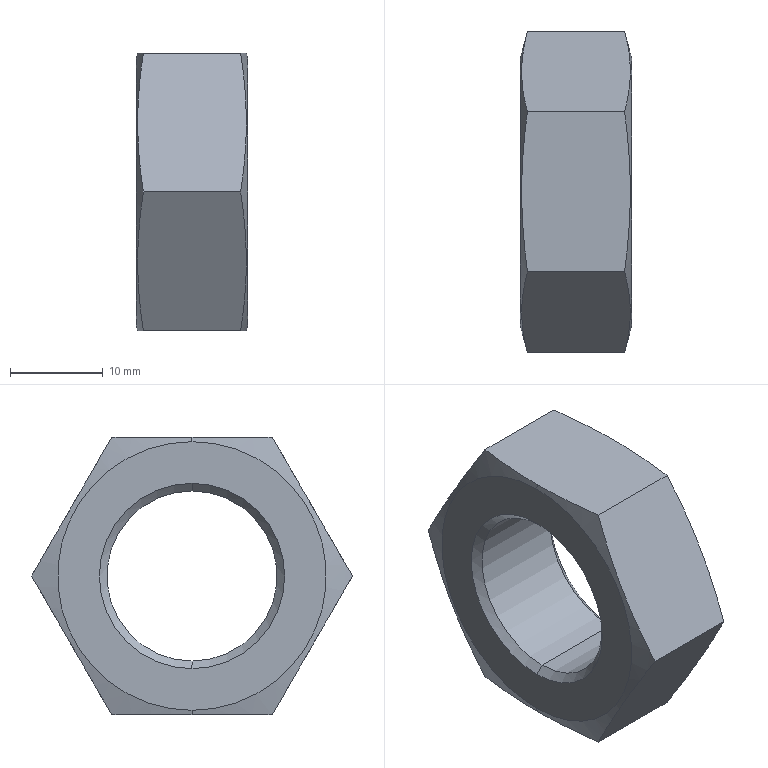Part | SolidWorks | features BaseBody 1 | 1 solid | 18 faces | box 12 x 34.641 x 30 mm | volume 6078 mm3 | cone 8 | plane 8 | cylinder 2 | commonest cylinder face diameters 18.376 x2
STEP:
#1=CARTESIAN_POINT('',(5.188,0.,9.188));
#2=VERTEX_POINT('',#1);
#3=CARTESIAN_POINT('',(5.188,0.,-9.188));
#4=VERTEX_POINT('',#3);
#5=CARTESIAN_POINT('',(5.188,0.,0.));
#6=DIRECTION('',(1.,0.,0.));
#7=DIRECTION('',(0.,0.,-1.));
#8=AXIS2_PLACEMENT_3D('',#5,#6,#7);
#9=CIRCLE('',#8,9.188);
#10=EDGE_CURVE('',#2,#4,#9,.T.);
#11=ORIENTED_EDGE('',*,*,#10,.F.);
#12=CARTESIAN_POINT('',(6.,0.,10.));
#13=VERTEX_POINT('',#12);
#14=CARTESIAN_POINT('',(6.,0.,10.));
#15=DIRECTION('',(0.7071,0.,0.7071));
#16=VECTOR('',#15,1000.);
#17=LINE('',#14,#16);
#18=EDGE_CURVE('',#2,#13,#17,.T.);
#19=ORIENTED_EDGE('',*,*,#18,.T.);
#20=CARTESIAN_POINT('',(6.,0.,-10.));
#21=VERTEX_POINT('',#20);
#22=CARTESIAN_POINT('',(6.,0.,0.));
#23=DIRECTION('',(1.,0.,0.));
#24=DIRECTION('',(0.,0.,-1.));
#25=AXIS2_PLACEMENT_3D('',#22,#23,#24);
#26=CIRCLE('',#25,10.);
#27=EDGE_CURVE('',#13,#21,#26,.T.);
#28=ORIENTED_EDGE('',*,*,#27,.T.);
#29=CARTESIAN_POINT('',(6.,0.,-10.));
#30=DIRECTION('',(0.7071,0.,-0.7071));
#31=VECTOR('',#30,1000.);
#32=LINE('',#29,#31);
#33=EDGE_CURVE('',#4,#21,#32,.T.);
#34=ORIENTED_EDGE('',*,*,#33,.F.);
#35=EDGE_LOOP('',(#11,#19,#28,#34));
#36=FACE_OUTER_BOUND('',#35,.T.);
#37=CARTESIAN_POINT('',(6.,0.,0.));
#38=DIRECTION('',(1.,0.,0.));
#39=DIRECTION('',(0.,0.,-1.));
#40=AXIS2_PLACEMENT_3D('',#37,#38,#39);
#41=CONICAL_SURFACE('',#40,10.,0.7854);
#42=ADVANCED_FACE('',(#36),#41,.F.);
#43=CARTESIAN_POINT('',(6.,0.,14.5));
#44=VERTEX_POINT('',#43);
#45=CARTESIAN_POINT('',(6.,0.,-14.5));
#46=VERTEX_POINT('',#45);
#47=CARTESIAN_POINT('',(6.,0.,0.));
#48=DIRECTION('',(-1.,0.,0.));
#49=DIRECTION('',(0.,0.,1.));
#50=AXIS2_PLACEMENT_3D('',#47,#48,#49);
#51=CIRCLE('',#50,14.5);
#52=EDGE_CURVE('',#44,#46,#51,.T.);
#53=ORIENTED_EDGE('',*,*,#52,.T.);
#54=CARTESIAN_POINT('',(5.866,0.,-15.));
#55=VERTEX_POINT('',#54);
#56=CARTESIAN_POINT('',(5.24,0.,-17.337));
#57=DIRECTION('',(-0.2588,0.,-0.9659));
#58=VECTOR('',#57,1000.);
#59=LINE('',#56,#58);
#60=EDGE_CURVE('',#46,#55,#59,.T.);
#61=ORIENTED_EDGE('',*,*,#60,.T.);
#62=CARTESIAN_POINT('',(5.244,8.66,-15.));
#63=VERTEX_POINT('',#62);
#64=CARTESIAN_POINT('',(5.866,0.,-15.));
#65=CARTESIAN_POINT('',(5.866,1.451,-15.));
#66=CARTESIAN_POINT('',(5.809,2.898,-15.));
#67=CARTESIAN_POINT('',(5.594,5.784,-15.));
#68=CARTESIAN_POINT('',(5.437,7.223,-15.));
#69=CARTESIAN_POINT('',(5.244,8.66,-15.));
#70=B_SPLINE_CURVE_WITH_KNOTS('',3,(#64,#65,#66,#67,#68,#69),.UNSPECIFIED.,.F.,.F.,(4,2,4),(0.,0.004341,0.008683),.UNSPECIFIED.);
#71=EDGE_CURVE('',#55,#63,#70,.T.);
#72=ORIENTED_EDGE('',*,*,#71,.T.);
#73=CARTESIAN_POINT('',(5.244,17.321,-0.000000051));
#74=VERTEX_POINT('',#73);
#75=CARTESIAN_POINT('',(5.244,8.66,-15.));
#76=CARTESIAN_POINT('',(5.438,9.382,-13.75));
#77=CARTESIAN_POINT('',(5.595,10.104,-12.5));
#78=CARTESIAN_POINT('',(5.809,11.547,-10.));
#79=CARTESIAN_POINT('',(5.923,12.99,-7.5));
#80=CARTESIAN_POINT('',(5.809,14.434,-5.));
#81=CARTESIAN_POINT('',(5.595,15.877,-2.5));
#82=CARTESIAN_POINT('',(5.438,16.599,-1.25));
#83=CARTESIAN_POINT('',(5.244,17.321,-0.000000051));
#84=B_SPLINE_CURVE_WITH_KNOTS('',3,(#75,#76,#77,#78,#79,#80,#81,#82,#83),.UNSPECIFIED.,.F.,.F.,(4,2,1,2,4),(0.,0.00433,0.00866,0.01299,0.01732),.UNSPECIFIED.);
#85=EDGE_CURVE('',#63,#74,#84,.T.);
#86=ORIENTED_EDGE('',*,*,#85,.T.);
#87=CARTESIAN_POINT('',(5.244,8.66,15.));
#88=VERTEX_POINT('',#87);
#89=CARTESIAN_POINT('',(5.244,17.321,-0.000000051));
#90=CARTESIAN_POINT('',(5.438,16.599,1.25));
#91=CARTESIAN_POINT('',(5.595,15.877,2.5));
#92=CARTESIAN_POINT('',(5.809,14.434,5.));
#93=CARTESIAN_POINT('',(5.923,12.99,7.5));
#94=CARTESIAN_POINT('',(5.809,11.547,10.));
#95=CARTESIAN_POINT('',(5.595,10.104,12.5));
#96=CARTESIAN_POINT('',(5.438,9.382,13.75));
#97=CARTESIAN_POINT('',(5.244,8.66,15.));
#98=B_SPLINE_CURVE_WITH_KNOTS('',3,(#89,#90,#91,#92,#93,#94,#95,#96,#97),.UNSPECIFIED.,.F.,.F.,(4,2,1,2,4),(0.,0.00433,0.00866,0.01299,0.01732),.UNSPECIFIED.);
#99=EDGE_CURVE('',#74,#88,#98,.T.);
#100=ORIENTED_EDGE('',*,*,#99,.T.);
#101=CARTESIAN_POINT('',(5.866,0.,15.));
#102=VERTEX_POINT('',#101);
#103=CARTESIAN_POINT('',(5.244,8.66,15.));
#104=CARTESIAN_POINT('',(5.437,7.223,15.));
#105=CARTESIAN_POINT('',(5.594,5.784,15.));
#106=CARTESIAN_POINT('',(5.809,2.898,15.));
#107=CARTESIAN_POINT('',(5.866,1.451,15.));
#108=CARTESIAN_POINT('',(5.866,0.,15.));
#109=B_SPLINE_CURVE_WITH_KNOTS('',3,(#103,#104,#105,#106,#107,#108),.UNSPECIFIED.,.F.,.F.,(4,2,4),(0.,0.004341,0.008683),.UNSPECIFIED.);
#110=EDGE_CURVE('',#88,#102,#109,.T.);
#111=ORIENTED_EDGE('',*,*,#110,.T.);
#112=CARTESIAN_POINT('',(5.24,0.,17.337));
#113=DIRECTION('',(-0.2588,0.,0.9659));
#114=VECTOR('',#113,1000.);
#115=LINE('',#112,#114);
#116=EDGE_CURVE('',#44,#102,#115,.T.);
#117=ORIENTED_EDGE('',*,*,#116,.F.);
#118=EDGE_LOOP('',(#53,#61,#72,#86,#100,#111,#117));
#119=FACE_OUTER_BOUND('',#118,.T.);
#120=CARTESIAN_POINT('',(5.24,0.,0.));
#121=DIRECTION('',(-1.,0.,0.));
#122=DIRECTION('',(0.,0.,1.));
#123=AXIS2_PLACEMENT_3D('',#120,#121,#122);
#124=CONICAL_SURFACE('',#123,17.337,1.309);
#125=ADVANCED_FACE('',(#119),#124,.T.);
#126=ORIENTED_EDGE('',*,*,#10,.T.);
#127=CARTESIAN_POINT('',(-5.188,0.,-9.188));
#128=VERTEX_POINT('',#127);
#129=CARTESIAN_POINT('',(6.,0.,-9.188));
#130=DIRECTION('',(-1.,0.,0.));
#131=VECTOR('',#130,1000.);
#132=LINE('',#129,#131);
#133=EDGE_CURVE('',#4,#128,#132,.T.);
#134=ORIENTED_EDGE('',*,*,#133,.T.);
#135=CARTESIAN_POINT('',(-5.188,0.,9.188));
#136=VERTEX_POINT('',#135);
#137=CARTESIAN_POINT('',(-5.188,0.,0.));
#138=DIRECTION('',(1.,0.,0.));
#139=DIRECTION('',(0.,0.,1.));
#140=AXIS2_PLACEMENT_3D('',#137,#138,#139);
#141=CIRCLE('',#140,9.188);
#142=EDGE_CURVE('',#136,#128,#141,.T.);
#143=ORIENTED_EDGE('',*,*,#142,.F.);
#144=CARTESIAN_POINT('',(6.,0.,9.188));
#145=DIRECTION('',(-1.,0.,0.));
#146=VECTOR('',#145,1000.);
#147=LINE('',#144,#146);
#148=EDGE_CURVE('',#2,#136,#147,.T.);
#149=ORIENTED_EDGE('',*,*,#148,.F.);
#150=EDGE_LOOP('',(#126,#134,#143,#149));
#151=FACE_OUTER_BOUND('',#150,.T.);
#152=CARTESIAN_POINT('',(6.,0.,0.));
#153=DIRECTION('',(-1.,0.,0.));
#154=DIRECTION('',(0.,0.,1.));
#155=AXIS2_PLACEMENT_3D('',#152,#153,#154);
#156=CYLINDRICAL_SURFACE('',#155,9.188);
#157=ADVANCED_FACE('',(#151),#156,.F.);
#158=ORIENTED_EDGE('',*,*,#142,.T.);
#159=CARTESIAN_POINT('',(-6.,0.,-10.));
#160=VERTEX_POINT('',#159);
#161=CARTESIAN_POINT('',(-6.,0.,-10.));
#162=DIRECTION('',(-0.7071,0.,-0.7071));
#163=VECTOR('',#162,1000.);
#164=LINE('',#161,#163);
#165=EDGE_CURVE('',#128,#160,#164,.T.);
#166=ORIENTED_EDGE('',*,*,#165,.T.);
#167=CARTESIAN_POINT('',(-6.,0.,10.));
#168=VERTEX_POINT('',#167);
#169=CARTESIAN_POINT('',(-6.,0.,0.));
#170=DIRECTION('',(1.,0.,0.));
#171=DIRECTION('',(0.,0.,1.));
#172=AXIS2_PLACEMENT_3D('',#169,#170,#171);
#173=CIRCLE('',#172,10.);
#174=EDGE_CURVE('',#168,#160,#173,.T.);
#175=ORIENTED_EDGE('',*,*,#174,.F.);
#176=CARTESIAN_POINT('',(-6.,0.,10.));
#177=DIRECTION('',(-0.7071,0.,0.7071));
#178=VECTOR('',#177,1000.);
#179=LINE('',#176,#178);
#180=EDGE_CURVE('',#136,#168,#179,.T.);
#181=ORIENTED_EDGE('',*,*,#180,.F.);
#182=EDGE_LOOP('',(#158,#166,#175,#181));
#183=FACE_OUTER_BOUND('',#182,.T.);
#184=CARTESIAN_POINT('',(-6.,0.,0.));
#185=DIRECTION('',(-1.,0.,0.));
#186=DIRECTION('',(0.,0.,1.));
#187=AXIS2_PLACEMENT_3D('',#184,#185,#186);
#188=CONICAL_SURFACE('',#187,10.,0.7854);
#189=ADVANCED_FACE('',(#183),#188,.F.);
#190=CARTESIAN_POINT('',(-6.,0.,-14.5));
#191=VERTEX_POINT('',#190);
#192=CARTESIAN_POINT('',(-6.,0.,14.5));
#193=VERTEX_POINT('',#192);
#194=CARTESIAN_POINT('',(-6.,0.,0.));
#195=DIRECTION('',(1.,0.,0.));
#196=DIRECTION('',(0.,0.,-1.));
#197=AXIS2_PLACEMENT_3D('',#194,#195,#196);
#198=CIRCLE('',#197,14.5);
#199=EDGE_CURVE('',#191,#193,#198,.T.);
#200=ORIENTED_EDGE('',*,*,#199,.T.);
#201=CARTESIAN_POINT('',(-5.866,0.,15.));
#202=VERTEX_POINT('',#201);
#203=CARTESIAN_POINT('',(-5.24,0.,17.337));
#204=DIRECTION('',(0.2588,0.,0.9659));
#205=VECTOR('',#204,1000.);
#206=LINE('',#203,#205);
#207=EDGE_CURVE('',#193,#202,#206,.T.);
#208=ORIENTED_EDGE('',*,*,#207,.T.);
#209=CARTESIAN_POINT('',(-5.244,8.66,15.));
#210=VERTEX_POINT('',#209);
#211=CARTESIAN_POINT('',(-5.866,0.,15.));
#212=CARTESIAN_POINT('',(-5.866,1.451,15.));
#213=CARTESIAN_POINT('',(-5.809,2.898,15.));
#214=CARTESIAN_POINT('',(-5.594,5.784,15.));
#215=CARTESIAN_POINT('',(-5.437,7.223,15.));
#216=CARTESIAN_POINT('',(-5.244,8.66,15.));
#217=B_SPLINE_CURVE_WITH_KNOTS('',3,(#211,#212,#213,#214,#215,#216),.UNSPECIFIED.,.F.,.F.,(4,2,4),(0.,0.004341,0.008683),.UNSPECIFIED.);
#218=EDGE_CURVE('',#202,#210,#217,.T.);
#219=ORIENTED_EDGE('',*,*,#218,.T.);
#220=CARTESIAN_POINT('',(-5.244,17.321,0.));
#221=VERTEX_POINT('',#220);
#222=CARTESIAN_POINT('',(-5.244,8.66,15.));
#223=CARTESIAN_POINT('',(-5.438,9.382,13.75));
#224=CARTESIAN_POINT('',(-5.595,10.104,12.5));
#225=CARTESIAN_POINT('',(-5.809,11.547,10.));
#226=CARTESIAN_POINT('',(-5.923,12.99,7.5));
#227=CARTESIAN_POINT('',(-5.809,14.434,5.));
#228=CARTESIAN_POINT('',(-5.595,15.877,2.5));
#229=CARTESIAN_POINT('',(-5.438,16.599,1.25));
#230=CARTESIAN_POINT('',(-5.244,17.321,0.));
#231=B_SPLINE_CURVE_WITH_KNOTS('',3,(#222,#223,#224,#225,#226,#227,#228,#229,#230),.UNSPECIFIED.,.F.,.F.,(4,2,1,2,4),(0.,0.00433,0.00866,0.01299,0.01732),.UNSPECIFIED.);
#232=EDGE_CURVE('',#210,#221,#231,.T.);
#233=ORIENTED_EDGE('',*,*,#232,.T.);
#234=CARTESIAN_POINT('',(-5.244,8.66,-15.));
#235=VERTEX_POINT('',#234);
#236=CARTESIAN_POINT('',(-5.244,17.321,0.));
#237=CARTESIAN_POINT('',(-5.438,16.599,-1.25));
#238=CARTESIAN_POINT('',(-5.595,15.877,-2.5));
#239=CARTESIAN_POINT('',(-5.809,14.434,-5.));
#240=CARTESIAN_POINT('',(-5.923,12.99,-7.5));
#241=CARTESIAN_POINT('',(-5.809,11.547,-10.));
#242=CARTESIAN_POINT('',(-5.595,10.104,-12.5));
#243=CARTESIAN_POINT('',(-5.438,9.382,-13.75));
#244=CARTESIAN_POINT('',(-5.244,8.66,-15.));
#245=B_SPLINE_CURVE_WITH_KNOTS('',3,(#236,#237,#238,#239,#240,#241,#242,#243,#244),.UNSPECIFIED.,.F.,.F.,(4,2,1,2,4),(0.,0.00433,0.00866,0.01299,0.01732),.UNSPECIFIED.);
#246=EDGE_CURVE('',#221,#235,#245,.T.);
#247=ORIENTED_EDGE('',*,*,#246,.T.);
#248=CARTESIAN_POINT('',(-5.866,0.,-15.));
#249=VERTEX_POINT('',#248);
#250=CARTESIAN_POINT('',(-5.244,8.66,-15.));
#251=CARTESIAN_POINT('',(-5.437,7.223,-15.));
#252=CARTESIAN_POINT('',(-5.594,5.784,-15.));
#253=CARTESIAN_POINT('',(-5.809,2.898,-15.));
#254=CARTESIAN_POINT('',(-5.866,1.451,-15.));
#255=CARTESIAN_POINT('',(-5.866,0.,-15.));
#256=B_SPLINE_CURVE_WITH_KNOTS('',3,(#250,#251,#252,#253,#254,#255),.UNSPECIFIED.,.F.,.F.,(4,2,4),(-0.008683,-0.004341,0.),.UNSPECIFIED.);
#257=EDGE_CURVE('',#235,#249,#256,.T.);
#258=ORIENTED_EDGE('',*,*,#257,.T.);
#259=CARTESIAN_POINT('',(-5.24,0.,-17.337));
#260=DIRECTION('',(0.2588,0.,-0.9659));
#261=VECTOR('',#260,1000.);
#262=LINE('',#259,#261);
#263=EDGE_CURVE('',#191,#249,#262,.T.);
#264=ORIENTED_EDGE('',*,*,#263,.F.);
#265=EDGE_LOOP('',(#200,#208,#219,#233,#247,#258,#264));
#266=FACE_OUTER_BOUND('',#265,.T.);
#267=CARTESIAN_POINT('',(-5.24,0.,0.));
#268=DIRECTION('',(1.,0.,0.));
#269=DIRECTION('',(0.,0.,-1.));
#270=AXIS2_PLACEMENT_3D('',#267,#268,#269);
#271=CONICAL_SURFACE('',#270,17.337,1.309);
#272=ADVANCED_FACE('',(#266),#271,.T.);
#273=CARTESIAN_POINT('',(6.,0.,0.));
#274=DIRECTION('',(1.,0.,0.));
#275=DIRECTION('',(0.,0.,-1.));
#276=AXIS2_PLACEMENT_3D('',#273,#274,#275);
#277=CIRCLE('',#276,10.);
#278=EDGE_CURVE('',#21,#13,#277,.T.);
#279=ORIENTED_EDGE('',*,*,#278,.F.);
#280=ORIENTED_EDGE('',*,*,#27,.F.);
#281=EDGE_LOOP('',(#279,#280));
#282=FACE_BOUND('',#281,.T.);
#283=ORIENTED_EDGE('',*,*,#52,.F.);
#284=CARTESIAN_POINT('',(6.,0.,0.));
#285=DIRECTION('',(-1.,0.,0.));
#286=DIRECTION('',(0.,0.,1.));
#287=AXIS2_PLACEMENT_3D('',#284,#285,#286);
#288=CIRCLE('',#287,14.5);
#289=EDGE_CURVE('',#46,#44,#288,.T.);
#290=ORIENTED_EDGE('',*,*,#289,.F.);
#291=EDGE_LOOP('',(#283,#290));
#292=FACE_OUTER_BOUND('',#291,.T.);
#293=CARTESIAN_POINT('',(6.,10.,0.));
#294=DIRECTION('',(-1.,0.,0.));
#295=DIRECTION('',(0.,0.,1.));
#296=AXIS2_PLACEMENT_3D('',#293,#294,#295);
#297=PLANE('',#296);
#298=ADVANCED_FACE('',(#282,#292),#297,.F.);
#299=ORIENTED_EDGE('',*,*,#18,.F.);
#300=CARTESIAN_POINT('',(5.188,0.,0.));
#301=DIRECTION('',(1.,0.,0.));
#302=DIRECTION('',(0.,0.,-1.));
#303=AXIS2_PLACEMENT_3D('',#300,#301,#302);
#304=CIRCLE('',#303,9.188);
#305=EDGE_CURVE('',#4,#2,#304,.T.);
#306=ORIENTED_EDGE('',*,*,#305,.F.);
#307=ORIENTED_EDGE('',*,*,#33,.T.);
#308=ORIENTED_EDGE('',*,*,#278,.T.);
#309=EDGE_LOOP('',(#299,#306,#307,#308));
#310=FACE_OUTER_BOUND('',#309,.T.);
#311=CARTESIAN_POINT('',(6.,0.,0.));
#312=DIRECTION('',(1.,0.,0.));
#313=DIRECTION('',(0.,0.,-1.));
#314=AXIS2_PLACEMENT_3D('',#311,#312,#313);
#315=CONICAL_SURFACE('',#314,10.,0.7854);
#316=ADVANCED_FACE('',(#310),#315,.F.);
#317=ORIENTED_EDGE('',*,*,#60,.F.);
#318=ORIENTED_EDGE('',*,*,#289,.T.);
#319=ORIENTED_EDGE('',*,*,#116,.T.);
#320=CARTESIAN_POINT('',(5.244,-8.66,15.));
#321=VERTEX_POINT('',#320);
#322=CARTESIAN_POINT('',(5.866,0.,15.));
#323=CARTESIAN_POINT('',(5.866,-1.451,15.));
#324=CARTESIAN_POINT('',(5.809,-2.898,15.));
#325=CARTESIAN_POINT('',(5.594,-5.784,15.));
#326=CARTESIAN_POINT('',(5.437,-7.223,15.));
#327=CARTESIAN_POINT('',(5.244,-8.66,15.));
#328=B_SPLINE_CURVE_WITH_KNOTS('',3,(#322,#323,#324,#325,#326,#327),.UNSPECIFIED.,.F.,.F.,(4,2,4),(0.008683,0.01302,0.01737),.UNSPECIFIED.);
#329=EDGE_CURVE('',#102,#321,#328,.T.);
#330=ORIENTED_EDGE('',*,*,#329,.T.);
#331=CARTESIAN_POINT('',(5.244,-17.321,0.000000051));
#332=VERTEX_POINT('',#331);
#333=CARTESIAN_POINT('',(5.244,-8.66,15.));
#334=CARTESIAN_POINT('',(5.438,-9.382,13.75));
#335=CARTESIAN_POINT('',(5.595,-10.104,12.5));
#336=CARTESIAN_POINT('',(5.809,-11.547,10.));
#337=CARTESIAN_POINT('',(5.923,-12.99,7.5));
#338=CARTESIAN_POINT('',(5.809,-14.434,5.));
#339=CARTESIAN_POINT('',(5.595,-15.877,2.5));
#340=CARTESIAN_POINT('',(5.438,-16.599,1.25));
#341=CARTESIAN_POINT('',(5.244,-17.321,0.000000051));
#342=B_SPLINE_CURVE_WITH_KNOTS('',3,(#333,#334,#335,#336,#337,#338,#339,#340,#341),.UNSPECIFIED.,.F.,.F.,(4,2,1,2,4),(0.,0.00433,0.00866,0.01299,0.01732),.UNSPECIFIED.);
#343=EDGE_CURVE('',#321,#332,#342,.T.);
#344=ORIENTED_EDGE('',*,*,#343,.T.);
#345=CARTESIAN_POINT('',(5.244,-8.66,-15.));
#346=VERTEX_POINT('',#345);
#347=CARTESIAN_POINT('',(5.244,-17.321,0.000000051));
#348=CARTESIAN_POINT('',(5.438,-16.599,-1.25));
#349=CARTESIAN_POINT('',(5.595,-15.877,-2.5));
#350=CARTESIAN_POINT('',(5.809,-14.434,-5.));
#351=CARTESIAN_POINT('',(5.923,-12.99,-7.5));
#352=CARTESIAN_POINT('',(5.809,-11.547,-10.));
#353=CARTESIAN_POINT('',(5.595,-10.104,-12.5));
#354=CARTESIAN_POINT('',(5.438,-9.382,-13.75));
#355=CARTESIAN_POINT('',(5.244,-8.66,-15.));
#356=B_SPLINE_CURVE_WITH_KNOTS('',3,(#347,#348,#349,#350,#351,#352,#353,#354,#355),.UNSPECIFIED.,.F.,.F.,(4,2,1,2,4),(0.,0.00433,0.00866,0.01299,0.01732),.UNSPECIFIED.);
#357=EDGE_CURVE('',#332,#346,#356,.T.);
#358=ORIENTED_EDGE('',*,*,#357,.T.);
#359=CARTESIAN_POINT('',(5.244,-8.66,-15.));
#360=CARTESIAN_POINT('',(5.437,-7.223,-15.));
#361=CARTESIAN_POINT('',(5.594,-5.784,-15.));
#362=CARTESIAN_POINT('',(5.809,-2.898,-15.));
#363=CARTESIAN_POINT('',(5.866,-1.451,-15.));
#364=CARTESIAN_POINT('',(5.866,0.,-15.));
#365=B_SPLINE_CURVE_WITH_KNOTS('',3,(#359,#360,#361,#362,#363,#364),.UNSPECIFIED.,.F.,.F.,(4,2,4),(-0.008683,-0.004341,0.),.UNSPECIFIED.);
#366=EDGE_CURVE('',#346,#55,#365,.T.);
#367=ORIENTED_EDGE('',*,*,#366,.T.);
#368=EDGE_LOOP('',(#317,#318,#319,#330,#344,#358,#367));
#369=FACE_OUTER_BOUND('',#368,.T.);
#370=CARTESIAN_POINT('',(5.24,0.,0.));
#371=DIRECTION('',(-1.,0.,0.));
#372=DIRECTION('',(0.,0.,1.));
#373=AXIS2_PLACEMENT_3D('',#370,#371,#372);
#374=CONICAL_SURFACE('',#373,17.337,1.309);
#375=ADVANCED_FACE('',(#369),#374,.T.);
#376=ORIENTED_EDGE('',*,*,#133,.F.);
#377=ORIENTED_EDGE('',*,*,#305,.T.);
#378=ORIENTED_EDGE('',*,*,#148,.T.);
#379=CARTESIAN_POINT('',(-5.188,0.,0.));
#380=DIRECTION('',(1.,0.,0.));
#381=DIRECTION('',(0.,0.,1.));
#382=AXIS2_PLACEMENT_3D('',#379,#380,#381);
#383=CIRCLE('',#382,9.188);
#384=EDGE_CURVE('',#128,#136,#383,.T.);
#385=ORIENTED_EDGE('',*,*,#384,.F.);
#386=EDGE_LOOP('',(#376,#377,#378,#385));
#387=FACE_OUTER_BOUND('',#386,.T.);
#388=CARTESIAN_POINT('',(6.,0.,0.));
#389=DIRECTION('',(-1.,0.,0.));
#390=DIRECTION('',(0.,0.,1.));
#391=AXIS2_PLACEMENT_3D('',#388,#389,#390);
#392=CYLINDRICAL_SURFACE('',#391,9.188);
#393=ADVANCED_FACE('',(#387),#392,.F.);
#394=CARTESIAN_POINT('',(-5.244,-8.66,15.));
#395=VERTEX_POINT('',#394);
#396=CARTESIAN_POINT('',(6.,-8.66,15.));
#397=DIRECTION('',(-1.,0.,0.));
#398=VECTOR('',#397,1000.);
#399=LINE('',#396,#398);
#400=EDGE_CURVE('',#321,#395,#399,.T.);
#401=ORIENTED_EDGE('',*,*,#400,.F.);
#402=ORIENTED_EDGE('',*,*,#329,.F.);
#403=ORIENTED_EDGE('',*,*,#110,.F.);
#404=CARTESIAN_POINT('',(6.,8.66,15.));
#405=DIRECTION('',(1.,0.,0.));
#406=VECTOR('',#405,1000.);
#407=LINE('',#404,#406);
#408=EDGE_CURVE('',#210,#88,#407,.T.);
#409=ORIENTED_EDGE('',*,*,#408,.F.);
#410=ORIENTED_EDGE('',*,*,#218,.F.);
#411=CARTESIAN_POINT('',(-5.244,-8.66,15.));
#412=CARTESIAN_POINT('',(-5.437,-7.223,15.));
#413=CARTESIAN_POINT('',(-5.594,-5.784,15.));
#414=CARTESIAN_POINT('',(-5.809,-2.898,15.));
#415=CARTESIAN_POINT('',(-5.866,-1.451,15.));
#416=CARTESIAN_POINT('',(-5.866,0.,15.));
#417=B_SPLINE_CURVE_WITH_KNOTS('',3,(#411,#412,#413,#414,#415,#416),.UNSPECIFIED.,.F.,.F.,(4,2,4),(-0.008683,-0.004341,0.),.UNSPECIFIED.);
#418=EDGE_CURVE('',#395,#202,#417,.T.);
#419=ORIENTED_EDGE('',*,*,#418,.F.);
#420=EDGE_LOOP('',(#401,#402,#403,#409,#410,#419));
#421=FACE_OUTER_BOUND('',#420,.T.);
#422=CARTESIAN_POINT('',(6.,8.66,15.));
#423=DIRECTION('',(0.,0.,-1.));
#424=DIRECTION('',(-1.,0.,0.));
#425=AXIS2_PLACEMENT_3D('',#422,#423,#424);
#426=PLANE('',#425);
#427=ADVANCED_FACE('',(#421),#426,.F.);
#428=ORIENTED_EDGE('',*,*,#99,.F.);
#429=CARTESIAN_POINT('',(6.,17.321,0.));
#430=DIRECTION('',(1.,0.,0.));
#431=VECTOR('',#430,1000.);
#432=LINE('',#429,#431);
#433=EDGE_CURVE('',#221,#74,#432,.T.);
#434=ORIENTED_EDGE('',*,*,#433,.F.);
#435=ORIENTED_EDGE('',*,*,#232,.F.);
#436=ORIENTED_EDGE('',*,*,#408,.T.);
#437=EDGE_LOOP('',(#428,#434,#435,#436));
#438=FACE_OUTER_BOUND('',#437,.T.);
#439=CARTESIAN_POINT('',(6.,17.321,0.));
#440=DIRECTION('',(0.,-0.866,-0.5));
#441=DIRECTION('',(0.,0.5,-0.866));
#442=AXIS2_PLACEMENT_3D('',#439,#440,#441);
#443=PLANE('',#442);
#444=ADVANCED_FACE('',(#438),#443,.F.);
#445=ORIENTED_EDGE('',*,*,#85,.F.);
#446=CARTESIAN_POINT('',(6.,8.66,-15.));
#447=DIRECTION('',(1.,0.,0.));
#448=VECTOR('',#447,1000.);
#449=LINE('',#446,#448);
#450=EDGE_CURVE('',#235,#63,#449,.T.);
#451=ORIENTED_EDGE('',*,*,#450,.F.);
#452=ORIENTED_EDGE('',*,*,#246,.F.);
#453=ORIENTED_EDGE('',*,*,#433,.T.);
#454=EDGE_LOOP('',(#445,#451,#452,#453));
#455=FACE_OUTER_BOUND('',#454,.T.);
#456=CARTESIAN_POINT('',(6.,8.66,-15.));
#457=DIRECTION('',(0.,-0.866,0.5));
#458=DIRECTION('',(0.,-0.5,-0.866));
#459=AXIS2_PLACEMENT_3D('',#456,#457,#458);
#460=PLANE('',#459);
#461=ADVANCED_FACE('',(#455),#460,.F.);
#462=ORIENTED_EDGE('',*,*,#366,.F.);
#463=CARTESIAN_POINT('',(-5.244,-8.66,-15.));
#464=VERTEX_POINT('',#463);
#465=CARTESIAN_POINT('',(6.,-8.66,-15.));
#466=DIRECTION('',(1.,0.,0.));
#467=VECTOR('',#466,1000.);
#468=LINE('',#465,#467);
#469=EDGE_CURVE('',#464,#346,#468,.T.);
#470=ORIENTED_EDGE('',*,*,#469,.F.);
#471=CARTESIAN_POINT('',(-5.866,0.,-15.));
#472=CARTESIAN_POINT('',(-5.866,-1.451,-15.));
#473=CARTESIAN_POINT('',(-5.809,-2.898,-15.));
#474=CARTESIAN_POINT('',(-5.594,-5.784,-15.));
#475=CARTESIAN_POINT('',(-5.437,-7.223,-15.));
#476=CARTESIAN_POINT('',(-5.244,-8.66,-15.));
#477=B_SPLINE_CURVE_WITH_KNOTS('',3,(#471,#472,#473,#474,#475,#476),.UNSPECIFIED.,.F.,.F.,(4,2,4),(0.,0.004341,0.008683),.UNSPECIFIED.);
#478=EDGE_CURVE('',#249,#464,#477,.T.);
#479=ORIENTED_EDGE('',*,*,#478,.F.);
#480=ORIENTED_EDGE('',*,*,#257,.F.);
#481=ORIENTED_EDGE('',*,*,#450,.T.);
#482=ORIENTED_EDGE('',*,*,#71,.F.);
#483=EDGE_LOOP('',(#462,#470,#479,#480,#481,#482));
#484=FACE_OUTER_BOUND('',#483,.T.);
#485=CARTESIAN_POINT('',(6.,-8.66,-15.));
#486=DIRECTION('',(0.,0.,1.));
#487=DIRECTION('',(1.,0.,0.));
#488=AXIS2_PLACEMENT_3D('',#485,#486,#487);
#489=PLANE('',#488);
#490=ADVANCED_FACE('',(#484),#489,.F.);
#491=ORIENTED_EDGE('',*,*,#357,.F.);
#492=CARTESIAN_POINT('',(-5.244,-17.321,0.));
#493=VERTEX_POINT('',#492);
#494=CARTESIAN_POINT('',(6.,-17.321,0.));
#495=DIRECTION('',(1.,0.,0.));
#496=VECTOR('',#495,1000.);
#497=LINE('',#494,#496);
#498=EDGE_CURVE('',#493,#332,#497,.T.);
#499=ORIENTED_EDGE('',*,*,#498,.F.);
#500=CARTESIAN_POINT('',(-5.244,-8.66,-15.));
#501=CARTESIAN_POINT('',(-5.438,-9.382,-13.75));
#502=CARTESIAN_POINT('',(-5.595,-10.104,-12.5));
#503=CARTESIAN_POINT('',(-5.809,-11.547,-10.));
#504=CARTESIAN_POINT('',(-5.923,-12.99,-7.5));
#505=CARTESIAN_POINT('',(-5.809,-14.434,-5.));
#506=CARTESIAN_POINT('',(-5.595,-15.877,-2.5));
#507=CARTESIAN_POINT('',(-5.438,-16.599,-1.25));
#508=CARTESIAN_POINT('',(-5.244,-17.321,0.));
#509=B_SPLINE_CURVE_WITH_KNOTS('',3,(#500,#501,#502,#503,#504,#505,#506,#507,#508),.UNSPECIFIED.,.F.,.F.,(4,2,1,2,4),(0.,0.00433,0.00866,0.01299,0.01732),.UNSPECIFIED.);
#510=EDGE_CURVE('',#464,#493,#509,.T.);
#511=ORIENTED_EDGE('',*,*,#510,.F.);
#512=ORIENTED_EDGE('',*,*,#469,.T.);
#513=EDGE_LOOP('',(#491,#499,#511,#512));
#514=FACE_OUTER_BOUND('',#513,.T.);
#515=CARTESIAN_POINT('',(6.,-17.321,0.));
#516=DIRECTION('',(0.,0.866,0.5));
#517=DIRECTION('',(0.,-0.5,0.866));
#518=AXIS2_PLACEMENT_3D('',#515,#516,#517);
#519=PLANE('',#518);
#520=ADVANCED_FACE('',(#514),#519,.F.);
#521=ORIENTED_EDGE('',*,*,#343,.F.);
#522=ORIENTED_EDGE('',*,*,#400,.T.);
#523=CARTESIAN_POINT('',(-5.244,-17.321,0.));
#524=CARTESIAN_POINT('',(-5.438,-16.599,1.25));
#525=CARTESIAN_POINT('',(-5.595,-15.877,2.5));
#526=CARTESIAN_POINT('',(-5.809,-14.434,5.));
#527=CARTESIAN_POINT('',(-5.923,-12.99,7.5));
#528=CARTESIAN_POINT('',(-5.809,-11.547,10.));
#529=CARTESIAN_POINT('',(-5.595,-10.104,12.5));
#530=CARTESIAN_POINT('',(-5.438,-9.382,13.75));
#531=CARTESIAN_POINT('',(-5.244,-8.66,15.));
#532=B_SPLINE_CURVE_WITH_KNOTS('',3,(#523,#524,#525,#526,#527,#528,#529,#530,#531),.UNSPECIFIED.,.F.,.F.,(4,2,1,2,4),(0.,0.00433,0.00866,0.01299,0.01732),.UNSPECIFIED.);
#533=EDGE_CURVE('',#493,#395,#532,.T.);
#534=ORIENTED_EDGE('',*,*,#533,.F.);
#535=ORIENTED_EDGE('',*,*,#498,.T.);
#536=EDGE_LOOP('',(#521,#522,#534,#535));
#537=FACE_OUTER_BOUND('',#536,.T.);
#538=CARTESIAN_POINT('',(6.,-8.66,15.));
#539=DIRECTION('',(0.,0.866,-0.5));
#540=DIRECTION('',(0.,0.5,0.866));
#541=AXIS2_PLACEMENT_3D('',#538,#539,#540);
#542=PLANE('',#541);
#543=ADVANCED_FACE('',(#537),#542,.F.);
#544=ORIENTED_EDGE('',*,*,#165,.F.);
#545=ORIENTED_EDGE('',*,*,#384,.T.);
#546=ORIENTED_EDGE('',*,*,#180,.T.);
#547=CARTESIAN_POINT('',(-6.,0.,0.));
#548=DIRECTION('',(1.,0.,0.));
#549=DIRECTION('',(0.,0.,1.));
#550=AXIS2_PLACEMENT_3D('',#547,#548,#549);
#551=CIRCLE('',#550,10.);
#552=EDGE_CURVE('',#160,#168,#551,.T.);
#553=ORIENTED_EDGE('',*,*,#552,.F.);
#554=EDGE_LOOP('',(#544,#545,#546,#553));
#555=FACE_OUTER_BOUND('',#554,.T.);
#556=CARTESIAN_POINT('',(-6.,0.,0.));
#557=DIRECTION('',(-1.,0.,0.));
#558=DIRECTION('',(0.,0.,1.));
#559=AXIS2_PLACEMENT_3D('',#556,#557,#558);
#560=CONICAL_SURFACE('',#559,10.,0.7854);
#561=ADVANCED_FACE('',(#555),#560,.F.);
#562=ORIENTED_EDGE('',*,*,#207,.F.);
#563=CARTESIAN_POINT('',(-6.,0.,0.));
#564=DIRECTION('',(1.,0.,0.));
#565=DIRECTION('',(0.,0.,-1.));
#566=AXIS2_PLACEMENT_3D('',#563,#564,#565);
#567=CIRCLE('',#566,14.5);
#568=EDGE_CURVE('',#193,#191,#567,.T.);
#569=ORIENTED_EDGE('',*,*,#568,.T.);
#570=ORIENTED_EDGE('',*,*,#263,.T.);
#571=ORIENTED_EDGE('',*,*,#478,.T.);
#572=ORIENTED_EDGE('',*,*,#510,.T.);
#573=ORIENTED_EDGE('',*,*,#533,.T.);
#574=ORIENTED_EDGE('',*,*,#418,.T.);
#575=EDGE_LOOP('',(#562,#569,#570,#571,#572,#573,#574));
#576=FACE_OUTER_BOUND('',#575,.T.);
#577=CARTESIAN_POINT('',(-5.24,0.,0.));
#578=DIRECTION('',(1.,0.,0.));
#579=DIRECTION('',(0.,0.,-1.));
#580=AXIS2_PLACEMENT_3D('',#577,#578,#579);
#581=CONICAL_SURFACE('',#580,17.337,1.309);
#582=ADVANCED_FACE('',(#576),#581,.T.);
#583=ORIENTED_EDGE('',*,*,#199,.F.);
#584=ORIENTED_EDGE('',*,*,#568,.F.);
#585=EDGE_LOOP('',(#583,#584));
#586=FACE_OUTER_BOUND('',#585,.T.);
#587=ORIENTED_EDGE('',*,*,#174,.T.);
#588=ORIENTED_EDGE('',*,*,#552,.T.);
#589=EDGE_LOOP('',(#587,#588));
#590=FACE_BOUND('',#589,.T.);
#591=CARTESIAN_POINT('',(-6.,14.5,0.));
#592=DIRECTION('',(1.,0.,0.));
#593=DIRECTION('',(0.,0.,-1.));
#594=AXIS2_PLACEMENT_3D('',#591,#592,#593);
#595=PLANE('',#594);
#596=ADVANCED_FACE('',(#586,#590),#595,.F.);
#597=CLOSED_SHELL('',(#42,#125,#157,#189,#272,#298,#316,#375,#393,#427,#444,#461,#490,#520,#543,#561,#582,#596));
#598=MANIFOLD_SOLID_BREP('',#597);
#599=CARTESIAN_POINT('',(0.,0.,0.));
#600=DIRECTION('',(0.,0.,1.));
#601=DIRECTION('',(1.,0.,0.));
#602=AXIS2_PLACEMENT_3D('',#599,#600,#601);
#603=(LENGTH_UNIT()NAMED_UNIT(*)SI_UNIT(.MILLI.,.METRE.));
#604=UNCERTAINTY_MEASURE_WITH_UNIT(LENGTH_MEASURE(0.00001),#603,'','');
#605=(NAMED_UNIT(*)PLANE_ANGLE_UNIT()SI_UNIT($,.RADIAN.));
#606=(NAMED_UNIT(*)SI_UNIT($,.STERADIAN.)SOLID_ANGLE_UNIT());
#607=(GEOMETRIC_REPRESENTATION_CONTEXT(3)GLOBAL_UNCERTAINTY_ASSIGNED_CONTEXT((#604))GLOBAL_UNIT_ASSIGNED_CONTEXT((#603,#605,#606))REPRESENTATION_CONTEXT('',''));
#608=ADVANCED_BREP_SHAPE_REPRESENTATION('',(#598,#602),#607);